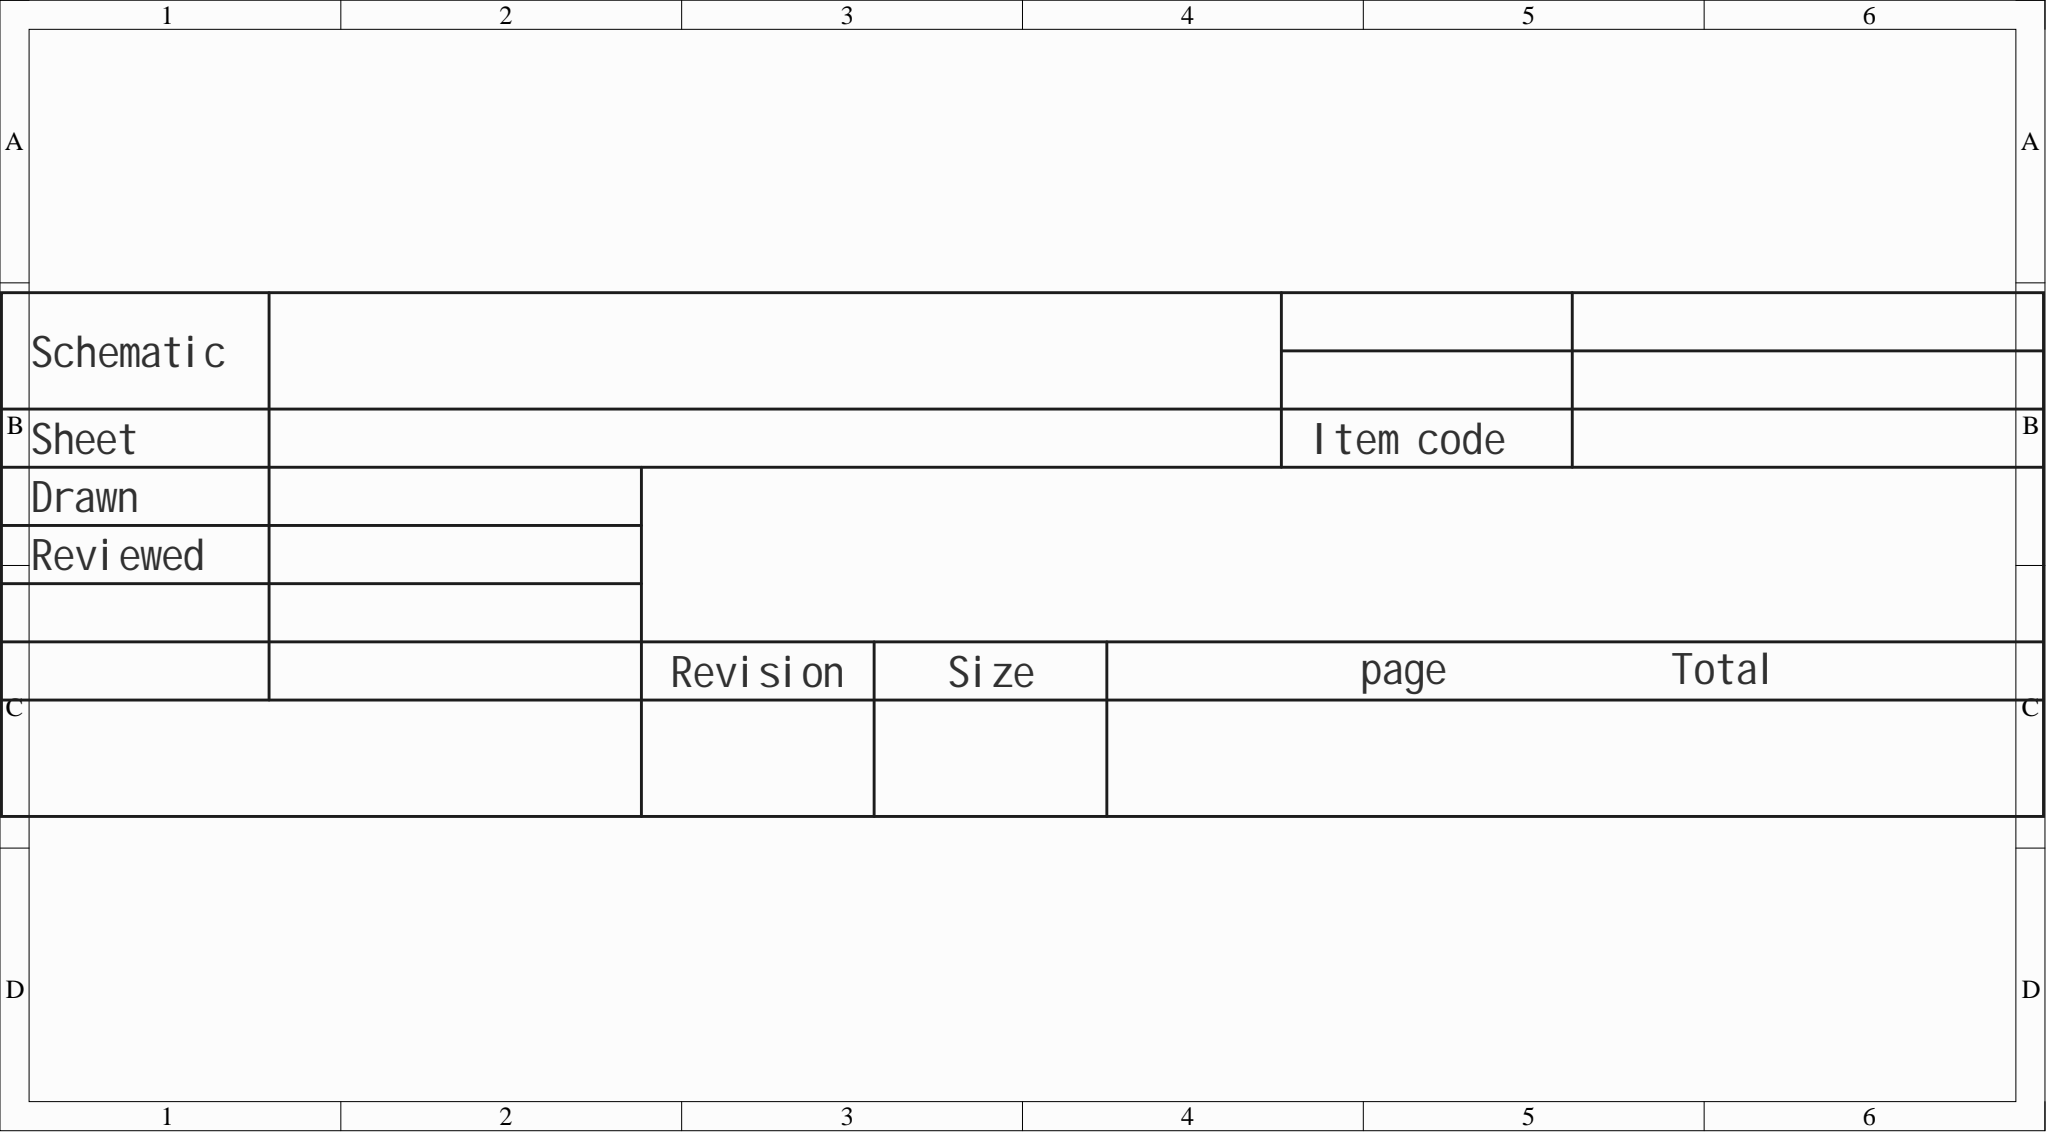Circuit board | Altium Designer | 38 parts | 28 nets
Bill of materials:
Comment,Description,Designator,Footprint,LibRef,Quantity
"1nF","","C1, C4, C5, C6","C0805","CAP_0805","4"
"0.01uF","","C2","C0805","CAP_0805","1"
"10nF","","C3","C0805","CAP_0805","1"
"0.11nF","","C12","C0805","CAP_0805","1"
"0.1nF","","C13","C0805","CAP_0805","1"
"","","H2","HDR-TH_2P-P2.54-V-M-1","HDR-M_2.54_1x2P","1"
"","","H3","HDR-TH_5P-P2.54-V-M","HDR-M_2.54_1x5P","1"
"","","H4","HDR-TH_1P-V-M_XKB_X4611WV-01I-C28D40","HDR-M_2.54_1x1P","1"
"510","","R1","R0603","Res_0603","1"
"60","","R2","R0603","Res_0603","1"
"24K","","R3","R_3296","R_3296","1"
"1K","","R4, R5, R15, R22","R0603","Res_0603","4"
"200","","R6","R0603","Res_0603","1"
"540","","R7","R0603","Res_0603","1"
"12k","","R8","R0603","Res_0603","1"
"100","","R9","R0603","Res_0603","1"
"480","","R10","R0603","Res_0603","1"
"120","","R11","R0603","Res_0603","1"
"300","","R12","R0603","Res_0603","1"
"1.8K","","R13","R0603","Res_0603","1"
"10k","","R14","R0603","Res_0603","1"
"400","","R16","R0603","Res_0603","1"
"16.5k","","R17","R0603","Res_0603","1"
"3.6k","","R18","R0603","Res_0603","1"
"720","","R19","R0603","Res_0603","1"
"1.35k","","R20","R0603","Res_0603","1"
"41k","","R21","R0603","Res_0603","1"
"50","","R23","R0603","Res_0603","1"
"90k","","R24","R0603","Res_0603","1"
"SN74LS74AN","Type: D-type; supply voltage: 4.75V~5.25V; clock frequency: 33MHz; number of elements: 2; bits per element: 1; max propagation delay: 25ns@2.5V,15pF; quiescent current (Iq): 8mA;","U2","PDIP-14_L19.5-W6.7-P2.54-LS7.9-BL","SN74LS74AN","1"
"LM324AD","Amplifier count: quad; gain-bandwidth product (GBP): 1.3MHz; input bias current (Ib): 15nA; slew rate (SR): 0.5V/us; bandwidth (-3db): -;","U7","SOIC-14_L8.7-W3.9-P1.27-LS6.0-BL","LM324AD","1"
"NE555PE4","Single-precision timer 8-PDIP 0 to 70","U8","PDIP-8_L9.6-W6.4-P2.54-LS7.9-BL-1","NE555PE4","1"
Netlist (Protel format):
[
C1
C0805
1nF



]
[
C2
C0805
0.01uF



]
[
C3
C0805
10nF



]
[
C4
C0805
1nF



]
[
C5
C0805
1nF



]
[
C6
C0805
1nF



]
[
C12
C0805
0.11nF



]
[
C13
C0805
0.1nF



]
[
H2
HDR-TH_2P-P2.54-V-M-1




]
[
H3
HDR-TH_5P-P2.54-V-M




]
[
H4
HDR-TH_1P-V-M_XKB_X4611WV-01I-C28D40




]
[
R1
R0603
510



]
[
R2
R0603
60



]
[
R3
R_3296
24K



]
[
R4
R0603
1K



]
[
R5
R0603
1K



]
[
R6
R0603
200



]
[
R7
R0603
540



]
[
R8
R0603
12k



]
[
R9
R0603
100



]
[
R10
R0603
480



]
[
R11
R0603
120



]
[
R12
R0603
300



]
[
R13
R0603
1.8K



]
[
R14
R0603
10k



]
[
R15
R0603
1K



]
[
R16
R0603
400



]
[
R17
R0603
16.5k



]
[
R18
R0603
3.6k



]
[
R19
R0603
720



]
[
R20
R0603
1.35k



]
[
R21
R0603
41k



]
[
R22
R0603
1k



]
[
R23
R0603
50



]
[
R24
R0603
90k



]
[
U2
PDIP-14_L19.5-W6.7-P2.54-LS7.9-BL
SN74LS74AN



]
[
U7
SOIC-14_L8.7-W3.9-P1.27-LS6.0-BL
LM324AD



]
[
U8
PDIP-8_L9.6-W6.4-P2.54-LS7.9-BL-1
NE555PE4



]
(
VCC
H2-1
R1-2
R5-2
R12-1
R22-1
U7-4
U8-4
U8-8
)
(
NetU2_8
U2-8
U2-12
)
(
NetU2_5
U2-5
U2-11
)
(
NetU2_2
U2-2
U2-6
)
(
NetR20_1
R20-1
R22-2
U7-12
)
(
NetR18_1
R18-1
R19-2
U7-9
)
(
NetR15_1
R15-1
U7-3
)
(
NetR10_2
R10-2
R13-2
U2-9
)
(
NetR9_1
R9-1
R12-2
R15-2
)
(
NetR7_2
R7-2
R14-2
R21-2
U2-3
U8-3
)
(
NetR4_2
R4-2
R5-1
U2-14
)
(
NetR3_2
R3-2
R8-1
)
(
NetR1_1
R1-1
R8-2
U8-7
)
(
NetC12_2
C12-2
C13-2
R21-1
R23-1
)
(
NetC12_1
C12-1
R24-1
U7-13
)
(
NetC6_2
C6-2
C13-1
R24-2
U7-14
)
(
NetC5_2
C5-2
R17-1
U7-10
)
(
NetC4_1
C4-1
R14-1
R17-2
)
(
NetC3_2
C3-2
R13-1
U7-2
)
(
NetC3_1
C3-1
R16-2
U7-1
)
(
NetC2_2
C2-2
U8-5
)
(
NetC1_2
C1-2
R3-1
U8-2
U8-6
)
(
GND
C1-1
C2-1
C5-1
H2-2
H4-1
R2-1
R4-1
R6-1
R9-2
R11-1
R18-2
R20-2
R23-2
U2-7
U7-11
U8-1
)
(
D
C4-2
H3-2
R19-1
U7-8
)
(
C
H3-5
R6-2
R16-1
)
(
B
H3-4
R10-1
R11-2
)
(
A2
C6-1
H3-3
)
(
A1
H3-1
R2-2
R7-1
)